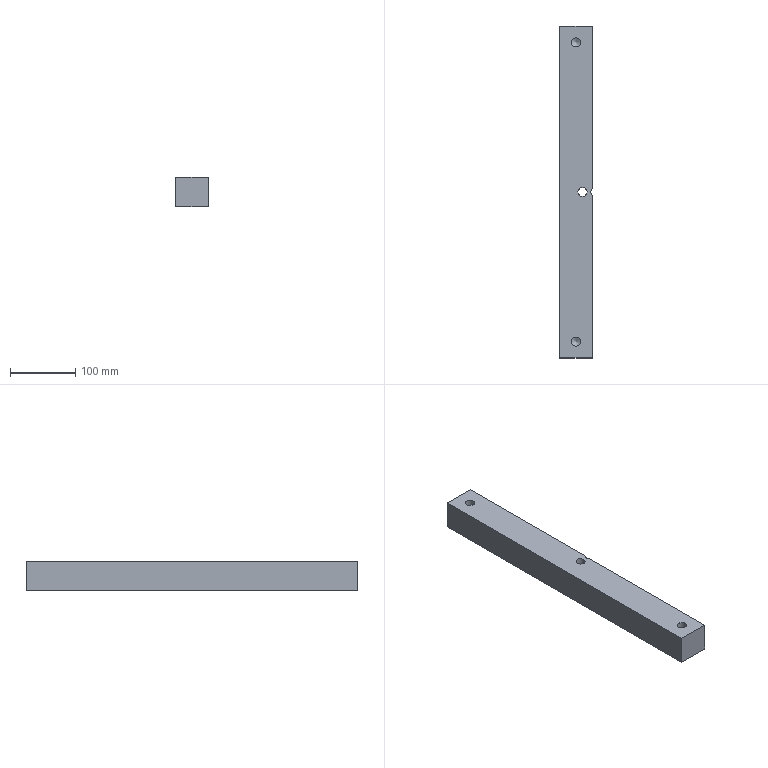Part | STEP file | 013_id2194_x_t | 1 solid | 13 faces | box 50 x 510 x 45 mm | volume 1133560 mm3 | plane 7 | cylinder 4 | cone 2 | commonest cylinder face diameters 14 x4
STEP:
#1=CARTESIAN_POINT('',(0.,0.,0.));
#2=DIRECTION('',(0.,0.,1.));
#3=DIRECTION('',(1.,0.,0.));
#4=AXIS2_PLACEMENT_3D('',#1,#2,#3);
#5=CARTESIAN_POINT('',(-701.5,-4.899,185.));
#6=VERTEX_POINT('',#5);
#7=CARTESIAN_POINT('',(-701.5,4.899,185.));
#8=VERTEX_POINT('',#7);
#9=CARTESIAN_POINT('',(-696.5,0.,185.));
#10=DIRECTION('',(0.,0.,-1.));
#11=DIRECTION('',(1.,0.,0.));
#12=AXIS2_PLACEMENT_3D('',#9,#10,#11);
#13=CIRCLE('',#12,7.);
#14=CARTESIAN_POINT('',(-751.5,-350.,185.));
#15=DIRECTION('',(0.,0.,1.));
#16=DIRECTION('',(0.,-1.,0.));
#17=AXIS2_PLACEMENT_3D('',#14,#15,#16);
#18=PLANE('',#17);
#19=CARTESIAN_POINT('',(-350.,62.));
#20=CARTESIAN_POINT('',(-337.876,62.));
#21=CARTESIAN_POINT('',(-343.938,51.5));
#22=CARTESIAN_POINT('',(-350.,41.));
#23=CARTESIAN_POINT('',(-356.062,51.5));
#24=CARTESIAN_POINT('',(-362.124,62.));
#25=CARTESIAN_POINT('',(-350.,62.));
#26=(BOUNDED_CURVE()B_SPLINE_CURVE(2,(#19,#20,#21,#22,#23,#24,#25),.UNSPECIFIED.,.T.,.F.)B_SPLINE_CURVE_WITH_KNOTS((1,2,2,2,2,1),(-2.094,0.,2.094,4.189,6.283,8.378),.UNSPECIFIED.)CURVE()GEOMETRIC_REPRESENTATION_ITEM()RATIONAL_B_SPLINE_CURVE((1.,0.5,1.,0.5,1.,0.5,1.))REPRESENTATION_ITEM(''));
#27=(GEOMETRIC_REPRESENTATION_CONTEXT(2)PARAMETRIC_REPRESENTATION_CONTEXT()REPRESENTATION_CONTEXT('',''));
#28=DEFINITIONAL_REPRESENTATION('',(#26),#27);
#29=PCURVE('',#18,#28);
#30=CARTESIAN_POINT('',(-696.5,0.,595.));
#31=DIRECTION('',(0.,0.,-1.));
#32=DIRECTION('',(-1.,0.,0.));
#33=AXIS2_PLACEMENT_3D('',#30,#31,#32);
#34=CYLINDRICAL_SURFACE('',#33,7.);
#35=CARTESIAN_POINT('',(-3.142,410.));
#36=DIRECTION('',(1.,0.));
#37=VECTOR('',#36,1.);
#38=LINE('',#35,#37);
#39=(GEOMETRIC_REPRESENTATION_CONTEXT(2)PARAMETRIC_REPRESENTATION_CONTEXT()REPRESENTATION_CONTEXT('',''));
#40=DEFINITIONAL_REPRESENTATION('',(#38),#39);
#41=PCURVE('',#34,#40);
#42=SURFACE_CURVE('',#13,(#29,#41),.PCURVE_S1.);
#43=EDGE_CURVE('',#6,#8,#42,.T.);
#44=ORIENTED_EDGE('',*,*,#43,.F.);
#45=CARTESIAN_POINT('',(-701.5,-255.,185.));
#46=VERTEX_POINT('',#45);
#47=CARTESIAN_POINT('',(-701.5,-350.,185.));
#48=DIRECTION('',(0.,1.,0.));
#49=VECTOR('',#48,1.);
#50=LINE('',#47,#49);
#51=CARTESIAN_POINT('',(0.,50.));
#52=DIRECTION('',(-1.,0.));
#53=VECTOR('',#52,1.);
#54=LINE('',#51,#53);
#55=(GEOMETRIC_REPRESENTATION_CONTEXT(2)PARAMETRIC_REPRESENTATION_CONTEXT()REPRESENTATION_CONTEXT('',''));
#56=DEFINITIONAL_REPRESENTATION('',(#54),#55);
#57=PCURVE('',#18,#56);
#58=CARTESIAN_POINT('',(-701.5,-350.,428.5));
#59=DIRECTION('',(-1.,0.,0.));
#60=DIRECTION('',(0.,0.,-1.));
#61=AXIS2_PLACEMENT_3D('',#58,#59,#60);
#62=PLANE('',#61);
#63=CARTESIAN_POINT('',(243.5,0.));
#64=DIRECTION('',(0.,-1.));
#65=VECTOR('',#64,1.);
#66=LINE('',#63,#65);
#67=(GEOMETRIC_REPRESENTATION_CONTEXT(2)PARAMETRIC_REPRESENTATION_CONTEXT()REPRESENTATION_CONTEXT('',''));
#68=DEFINITIONAL_REPRESENTATION('',(#66),#67);
#69=PCURVE('',#62,#68);
#70=SURFACE_CURVE('',#50,(#57,#69),.PCURVE_S1.);
#71=EDGE_CURVE('',#46,#6,#70,.T.);
#72=ORIENTED_EDGE('',*,*,#71,.F.);
#73=CARTESIAN_POINT('',(-751.5,-255.,185.));
#74=VERTEX_POINT('',#73);
#75=CARTESIAN_POINT('',(-751.5,-255.,185.));
#76=DIRECTION('',(-1.,0.,0.));
#77=VECTOR('',#76,1.);
#78=LINE('',#75,#77);
#79=CARTESIAN_POINT('',(-95.,0.));
#80=DIRECTION('',(0.,-1.));
#81=VECTOR('',#80,1.);
#82=LINE('',#79,#81);
#83=(GEOMETRIC_REPRESENTATION_CONTEXT(2)PARAMETRIC_REPRESENTATION_CONTEXT()REPRESENTATION_CONTEXT('',''));
#84=DEFINITIONAL_REPRESENTATION('',(#82),#83);
#85=PCURVE('',#18,#84);
#86=CARTESIAN_POINT('',(-751.5,-255.,428.5));
#87=DIRECTION('',(0.,1.,0.));
#88=DIRECTION('',(0.,0.,1.));
#89=AXIS2_PLACEMENT_3D('',#86,#87,#88);
#90=PLANE('',#89);
#91=CARTESIAN_POINT('',(-243.5,0.));
#92=DIRECTION('',(0.,-1.));
#93=VECTOR('',#92,1.);
#94=LINE('',#91,#93);
#95=(GEOMETRIC_REPRESENTATION_CONTEXT(2)PARAMETRIC_REPRESENTATION_CONTEXT()REPRESENTATION_CONTEXT('',''));
#96=DEFINITIONAL_REPRESENTATION('',(#94),#95);
#97=PCURVE('',#90,#96);
#98=SURFACE_CURVE('',#78,(#85,#97),.PCURVE_S1.);
#99=EDGE_CURVE('',#46,#74,#98,.T.);
#100=ORIENTED_EDGE('',*,*,#99,.T.);
#101=CARTESIAN_POINT('',(-751.5,255.,185.));
#102=VERTEX_POINT('',#101);
#103=CARTESIAN_POINT('',(-751.5,-350.,185.));
#104=DIRECTION('',(0.,1.,0.));
#105=VECTOR('',#104,1.);
#106=LINE('',#103,#105);
#107=CARTESIAN_POINT('',(0.,0.));
#108=DIRECTION('',(-1.,0.));
#109=VECTOR('',#108,1.);
#110=LINE('',#107,#109);
#111=(GEOMETRIC_REPRESENTATION_CONTEXT(2)PARAMETRIC_REPRESENTATION_CONTEXT()REPRESENTATION_CONTEXT('',''));
#112=DEFINITIONAL_REPRESENTATION('',(#110),#111);
#113=PCURVE('',#18,#112);
#114=CARTESIAN_POINT('',(-751.5,-350.,428.5));
#115=DIRECTION('',(-1.,0.,0.));
#116=DIRECTION('',(0.,0.,-1.));
#117=AXIS2_PLACEMENT_3D('',#114,#115,#116);
#118=PLANE('',#117);
#119=CARTESIAN_POINT('',(243.5,0.));
#120=DIRECTION('',(0.,-1.));
#121=VECTOR('',#120,1.);
#122=LINE('',#119,#121);
#123=(GEOMETRIC_REPRESENTATION_CONTEXT(2)PARAMETRIC_REPRESENTATION_CONTEXT()REPRESENTATION_CONTEXT('',''));
#124=DEFINITIONAL_REPRESENTATION('',(#122),#123);
#125=PCURVE('',#118,#124);
#126=SURFACE_CURVE('',#106,(#113,#125),.PCURVE_S1.);
#127=EDGE_CURVE('',#74,#102,#126,.T.);
#128=ORIENTED_EDGE('',*,*,#127,.T.);
#129=CARTESIAN_POINT('',(-701.5,255.,185.));
#130=VERTEX_POINT('',#129);
#131=CARTESIAN_POINT('',(-751.5,255.,185.));
#132=DIRECTION('',(-1.,0.,0.));
#133=VECTOR('',#132,1.);
#134=LINE('',#131,#133);
#135=CARTESIAN_POINT('',(-605.,0.));
#136=DIRECTION('',(0.,-1.));
#137=VECTOR('',#136,1.);
#138=LINE('',#135,#137);
#139=(GEOMETRIC_REPRESENTATION_CONTEXT(2)PARAMETRIC_REPRESENTATION_CONTEXT()REPRESENTATION_CONTEXT('',''));
#140=DEFINITIONAL_REPRESENTATION('',(#138),#139);
#141=PCURVE('',#18,#140);
#142=CARTESIAN_POINT('',(-751.5,255.,428.5));
#143=DIRECTION('',(0.,1.,0.));
#144=DIRECTION('',(0.,0.,1.));
#145=AXIS2_PLACEMENT_3D('',#142,#143,#144);
#146=PLANE('',#145);
#147=CARTESIAN_POINT('',(-243.5,0.));
#148=DIRECTION('',(0.,-1.));
#149=VECTOR('',#148,1.);
#150=LINE('',#147,#149);
#151=(GEOMETRIC_REPRESENTATION_CONTEXT(2)PARAMETRIC_REPRESENTATION_CONTEXT()REPRESENTATION_CONTEXT('',''));
#152=DEFINITIONAL_REPRESENTATION('',(#150),#151);
#153=PCURVE('',#146,#152);
#154=SURFACE_CURVE('',#134,(#141,#153),.PCURVE_S1.);
#155=EDGE_CURVE('',#130,#102,#154,.T.);
#156=ORIENTED_EDGE('',*,*,#155,.F.);
#157=CARTESIAN_POINT('',(-701.5,-350.,185.));
#158=DIRECTION('',(0.,1.,0.));
#159=VECTOR('',#158,1.);
#160=LINE('',#157,#159);
#161=CARTESIAN_POINT('',(0.,50.));
#162=DIRECTION('',(-1.,0.));
#163=VECTOR('',#162,1.);
#164=LINE('',#161,#163);
#165=(GEOMETRIC_REPRESENTATION_CONTEXT(2)PARAMETRIC_REPRESENTATION_CONTEXT()REPRESENTATION_CONTEXT('',''));
#166=DEFINITIONAL_REPRESENTATION('',(#164),#165);
#167=PCURVE('',#18,#166);
#168=CARTESIAN_POINT('',(-701.5,-350.,428.5));
#169=DIRECTION('',(-1.,0.,0.));
#170=DIRECTION('',(0.,0.,-1.));
#171=AXIS2_PLACEMENT_3D('',#168,#169,#170);
#172=PLANE('',#171);
#173=CARTESIAN_POINT('',(243.5,0.));
#174=DIRECTION('',(0.,-1.));
#175=VECTOR('',#174,1.);
#176=LINE('',#173,#175);
#177=(GEOMETRIC_REPRESENTATION_CONTEXT(2)PARAMETRIC_REPRESENTATION_CONTEXT()REPRESENTATION_CONTEXT('',''));
#178=DEFINITIONAL_REPRESENTATION('',(#176),#177);
#179=PCURVE('',#172,#178);
#180=SURFACE_CURVE('',#160,(#167,#179),.PCURVE_S1.);
#181=EDGE_CURVE('',#8,#130,#180,.T.);
#182=ORIENTED_EDGE('',*,*,#181,.F.);
#183=EDGE_LOOP('',(#44,#72,#100,#128,#156,#182));
#184=FACE_BOUND('',#183,.T.);
#185=CARTESIAN_POINT('',(-709.5,0.,185.));
#186=VERTEX_POINT('',#185);
#187=CARTESIAN_POINT('',(-716.5,0.,185.));
#188=DIRECTION('',(0.,0.,-1.));
#189=DIRECTION('',(1.,0.,0.));
#190=AXIS2_PLACEMENT_3D('',#187,#188,#189);
#191=CIRCLE('',#190,7.);
#192=CARTESIAN_POINT('',(-350.,42.));
#193=CARTESIAN_POINT('',(-337.876,42.));
#194=CARTESIAN_POINT('',(-343.938,31.5));
#195=CARTESIAN_POINT('',(-350.,21.));
#196=CARTESIAN_POINT('',(-356.062,31.5));
#197=CARTESIAN_POINT('',(-362.124,42.));
#198=CARTESIAN_POINT('',(-350.,42.));
#199=(BOUNDED_CURVE()B_SPLINE_CURVE(2,(#192,#193,#194,#195,#196,#197,#198),.UNSPECIFIED.,.T.,.F.)B_SPLINE_CURVE_WITH_KNOTS((1,2,2,2,2,1),(-2.094,0.,2.094,4.189,6.283,8.378),.UNSPECIFIED.)CURVE()GEOMETRIC_REPRESENTATION_ITEM()RATIONAL_B_SPLINE_CURVE((1.,0.5,1.,0.5,1.,0.5,1.))REPRESENTATION_ITEM(''));
#200=(GEOMETRIC_REPRESENTATION_CONTEXT(2)PARAMETRIC_REPRESENTATION_CONTEXT()REPRESENTATION_CONTEXT('',''));
#201=DEFINITIONAL_REPRESENTATION('',(#199),#200);
#202=PCURVE('',#18,#201);
#203=CARTESIAN_POINT('',(-716.5,0.,595.));
#204=DIRECTION('',(0.,0.,-1.));
#205=DIRECTION('',(-1.,0.,0.));
#206=AXIS2_PLACEMENT_3D('',#203,#204,#205);
#207=CYLINDRICAL_SURFACE('',#206,7.);
#208=CARTESIAN_POINT('',(3.142,410.));
#209=DIRECTION('',(1.,0.));
#210=VECTOR('',#209,1.);
#211=LINE('',#208,#210);
#212=(GEOMETRIC_REPRESENTATION_CONTEXT(2)PARAMETRIC_REPRESENTATION_CONTEXT()REPRESENTATION_CONTEXT('',''));
#213=DEFINITIONAL_REPRESENTATION('',(#211),#212);
#214=PCURVE('',#207,#213);
#215=SURFACE_CURVE('',#191,(#202,#214),.PCURVE_S1.);
#216=EDGE_CURVE('',#186,#186,#215,.T.);
#217=ORIENTED_EDGE('',*,*,#216,.F.);
#218=EDGE_LOOP('',(#217));
#219=FACE_BOUND('',#218,.T.);
#220=ADVANCED_FACE('',(#184,#219),#18,.F.);
#221=CARTESIAN_POINT('',(-701.5,4.899,230.));
#222=VERTEX_POINT('',#221);
#223=CARTESIAN_POINT('',(-701.5,255.,230.));
#224=VERTEX_POINT('',#223);
#225=CARTESIAN_POINT('',(-701.5,-350.,230.));
#226=DIRECTION('',(0.,1.,0.));
#227=VECTOR('',#226,1.);
#228=LINE('',#225,#227);
#229=CARTESIAN_POINT('',(198.5,0.));
#230=DIRECTION('',(0.,-1.));
#231=VECTOR('',#230,1.);
#232=LINE('',#229,#231);
#233=(GEOMETRIC_REPRESENTATION_CONTEXT(2)PARAMETRIC_REPRESENTATION_CONTEXT()REPRESENTATION_CONTEXT('',''));
#234=DEFINITIONAL_REPRESENTATION('',(#232),#233);
#235=PCURVE('',#172,#234);
#236=CARTESIAN_POINT('',(-546.5,-140.,230.));
#237=DIRECTION('',(0.,0.,1.));
#238=DIRECTION('',(1.,0.,0.));
#239=AXIS2_PLACEMENT_3D('',#236,#237,#238);
#240=PLANE('',#239);
#241=CARTESIAN_POINT('',(-155.,-210.));
#242=DIRECTION('',(0.,1.));
#243=VECTOR('',#242,1.);
#244=LINE('',#241,#243);
#245=(GEOMETRIC_REPRESENTATION_CONTEXT(2)PARAMETRIC_REPRESENTATION_CONTEXT()REPRESENTATION_CONTEXT('',''));
#246=DEFINITIONAL_REPRESENTATION('',(#244),#245);
#247=PCURVE('',#240,#246);
#248=SURFACE_CURVE('',#228,(#235,#247),.PCURVE_S1.);
#249=EDGE_CURVE('',#222,#224,#248,.T.);
#250=ORIENTED_EDGE('',*,*,#249,.F.);
#251=CARTESIAN_POINT('',(-701.5,4.899,595.));
#252=DIRECTION('',(0.,0.,-1.));
#253=VECTOR('',#252,1.);
#254=LINE('',#251,#253);
#255=CARTESIAN_POINT('',(-166.5,-354.899));
#256=DIRECTION('',(1.,0.));
#257=VECTOR('',#256,1.);
#258=LINE('',#255,#257);
#259=(GEOMETRIC_REPRESENTATION_CONTEXT(2)PARAMETRIC_REPRESENTATION_CONTEXT()REPRESENTATION_CONTEXT('',''));
#260=DEFINITIONAL_REPRESENTATION('',(#258),#259);
#261=PCURVE('',#172,#260);
#262=CARTESIAN_POINT('',(0.7752,0.));
#263=DIRECTION('',(0.,1.));
#264=VECTOR('',#263,1.);
#265=LINE('',#262,#264);
#266=(GEOMETRIC_REPRESENTATION_CONTEXT(2)PARAMETRIC_REPRESENTATION_CONTEXT()REPRESENTATION_CONTEXT('',''));
#267=DEFINITIONAL_REPRESENTATION('',(#265),#266);
#268=PCURVE('',#34,#267);
#269=SURFACE_CURVE('',#254,(#261,#268),.PCURVE_S1.);
#270=EDGE_CURVE('',#222,#8,#269,.T.);
#271=ORIENTED_EDGE('',*,*,#270,.T.);
#272=ORIENTED_EDGE('',*,*,#181,.T.);
#273=CARTESIAN_POINT('',(-701.5,255.,428.5));
#274=DIRECTION('',(0.,0.,1.));
#275=VECTOR('',#274,1.);
#276=LINE('',#273,#275);
#277=CARTESIAN_POINT('',(0.,-605.));
#278=DIRECTION('',(-1.,0.));
#279=VECTOR('',#278,1.);
#280=LINE('',#277,#279);
#281=(GEOMETRIC_REPRESENTATION_CONTEXT(2)PARAMETRIC_REPRESENTATION_CONTEXT()REPRESENTATION_CONTEXT('',''));
#282=DEFINITIONAL_REPRESENTATION('',(#280),#281);
#283=PCURVE('',#172,#282);
#284=CARTESIAN_POINT('',(0.,50.));
#285=DIRECTION('',(1.,0.));
#286=VECTOR('',#285,1.);
#287=LINE('',#284,#286);
#288=(GEOMETRIC_REPRESENTATION_CONTEXT(2)PARAMETRIC_REPRESENTATION_CONTEXT()REPRESENTATION_CONTEXT('',''));
#289=DEFINITIONAL_REPRESENTATION('',(#287),#288);
#290=PCURVE('',#146,#289);
#291=SURFACE_CURVE('',#276,(#283,#290),.PCURVE_S1.);
#292=EDGE_CURVE('',#130,#224,#291,.T.);
#293=ORIENTED_EDGE('',*,*,#292,.T.);
#294=EDGE_LOOP('',(#250,#271,#272,#293));
#295=FACE_BOUND('',#294,.T.);
#296=ADVANCED_FACE('',(#295),#172,.F.);
#297=CARTESIAN_POINT('',(-709.5,0.,230.));
#298=VERTEX_POINT('',#297);
#299=CARTESIAN_POINT('',(-716.5,0.,230.));
#300=DIRECTION('',(0.,0.,1.));
#301=DIRECTION('',(1.,0.,0.));
#302=AXIS2_PLACEMENT_3D('',#299,#300,#301);
#303=CIRCLE('',#302,7.);
#304=CARTESIAN_POINT('',(-170.,140.));
#305=DIRECTION('',(1.,0.));
#306=AXIS2_PLACEMENT_2D('',#304,#305);
#307=CIRCLE('',#306,7.);
#308=(GEOMETRIC_REPRESENTATION_CONTEXT(2)PARAMETRIC_REPRESENTATION_CONTEXT()REPRESENTATION_CONTEXT('',''));
#309=DEFINITIONAL_REPRESENTATION('',(#307),#308);
#310=PCURVE('',#240,#309);
#311=CARTESIAN_POINT('',(9.425,365.));
#312=DIRECTION('',(-1.,0.));
#313=VECTOR('',#312,1.);
#314=LINE('',#311,#313);
#315=(GEOMETRIC_REPRESENTATION_CONTEXT(2)PARAMETRIC_REPRESENTATION_CONTEXT()REPRESENTATION_CONTEXT('',''));
#316=DEFINITIONAL_REPRESENTATION('',(#314),#315);
#317=PCURVE('',#207,#316);
#318=SURFACE_CURVE('',#303,(#310,#317),.PCURVE_S1.);
#319=EDGE_CURVE('',#298,#298,#318,.T.);
#320=ORIENTED_EDGE('',*,*,#319,.F.);
#321=EDGE_LOOP('',(#320));
#322=FACE_BOUND('',#321,.T.);
#323=CARTESIAN_POINT('',(-701.5,-4.899,230.));
#324=VERTEX_POINT('',#323);
#325=CARTESIAN_POINT('',(-696.5,0.,230.));
#326=DIRECTION('',(0.,0.,1.));
#327=DIRECTION('',(1.,0.,0.));
#328=AXIS2_PLACEMENT_3D('',#325,#326,#327);
#329=CIRCLE('',#328,7.);
#330=CARTESIAN_POINT('',(-150.,140.));
#331=DIRECTION('',(1.,0.));
#332=AXIS2_PLACEMENT_2D('',#330,#331);
#333=CIRCLE('',#332,7.);
#334=(GEOMETRIC_REPRESENTATION_CONTEXT(2)PARAMETRIC_REPRESENTATION_CONTEXT()REPRESENTATION_CONTEXT('',''));
#335=DEFINITIONAL_REPRESENTATION('',(#333),#334);
#336=PCURVE('',#240,#335);
#337=CARTESIAN_POINT('',(3.142,365.));
#338=DIRECTION('',(-1.,0.));
#339=VECTOR('',#338,1.);
#340=LINE('',#337,#339);
#341=(GEOMETRIC_REPRESENTATION_CONTEXT(2)PARAMETRIC_REPRESENTATION_CONTEXT()REPRESENTATION_CONTEXT('',''));
#342=DEFINITIONAL_REPRESENTATION('',(#340),#341);
#343=PCURVE('',#34,#342);
#344=SURFACE_CURVE('',#329,(#336,#343),.PCURVE_S1.);
#345=EDGE_CURVE('',#222,#324,#344,.T.);
#346=ORIENTED_EDGE('',*,*,#345,.F.);
#347=ORIENTED_EDGE('',*,*,#249,.T.);
#348=CARTESIAN_POINT('',(-751.5,255.,230.));
#349=VERTEX_POINT('',#348);
#350=CARTESIAN_POINT('',(-751.5,255.,230.));
#351=DIRECTION('',(-1.,0.,0.));
#352=VECTOR('',#351,1.);
#353=LINE('',#350,#352);
#354=CARTESIAN_POINT('',(-205.,395.));
#355=DIRECTION('',(-1.,0.));
#356=VECTOR('',#355,1.);
#357=LINE('',#354,#356);
#358=(GEOMETRIC_REPRESENTATION_CONTEXT(2)PARAMETRIC_REPRESENTATION_CONTEXT()REPRESENTATION_CONTEXT('',''));
#359=DEFINITIONAL_REPRESENTATION('',(#357),#358);
#360=PCURVE('',#240,#359);
#361=CARTESIAN_POINT('',(-198.5,0.));
#362=DIRECTION('',(0.,-1.));
#363=VECTOR('',#362,1.);
#364=LINE('',#361,#363);
#365=(GEOMETRIC_REPRESENTATION_CONTEXT(2)PARAMETRIC_REPRESENTATION_CONTEXT()REPRESENTATION_CONTEXT('',''));
#366=DEFINITIONAL_REPRESENTATION('',(#364),#365);
#367=PCURVE('',#146,#366);
#368=SURFACE_CURVE('',#353,(#360,#367),.PCURVE_S1.);
#369=EDGE_CURVE('',#224,#349,#368,.T.);
#370=ORIENTED_EDGE('',*,*,#369,.T.);
#371=CARTESIAN_POINT('',(-751.5,-255.,230.));
#372=VERTEX_POINT('',#371);
#373=CARTESIAN_POINT('',(-751.5,-350.,230.));
#374=DIRECTION('',(0.,-1.,0.));
#375=VECTOR('',#374,1.);
#376=LINE('',#373,#375);
#377=CARTESIAN_POINT('',(-205.,-210.));
#378=DIRECTION('',(0.,-1.));
#379=VECTOR('',#378,1.);
#380=LINE('',#377,#379);
#381=(GEOMETRIC_REPRESENTATION_CONTEXT(2)PARAMETRIC_REPRESENTATION_CONTEXT()REPRESENTATION_CONTEXT('',''));
#382=DEFINITIONAL_REPRESENTATION('',(#380),#381);
#383=PCURVE('',#240,#382);
#384=CARTESIAN_POINT('',(198.5,0.));
#385=DIRECTION('',(0.,1.));
#386=VECTOR('',#385,1.);
#387=LINE('',#384,#386);
#388=(GEOMETRIC_REPRESENTATION_CONTEXT(2)PARAMETRIC_REPRESENTATION_CONTEXT()REPRESENTATION_CONTEXT('',''));
#389=DEFINITIONAL_REPRESENTATION('',(#387),#388);
#390=PCURVE('',#118,#389);
#391=SURFACE_CURVE('',#376,(#383,#390),.PCURVE_S1.);
#392=EDGE_CURVE('',#349,#372,#391,.T.);
#393=ORIENTED_EDGE('',*,*,#392,.T.);
#394=CARTESIAN_POINT('',(-701.5,-255.,230.));
#395=VERTEX_POINT('',#394);
#396=CARTESIAN_POINT('',(-751.5,-255.,230.));
#397=DIRECTION('',(-1.,0.,0.));
#398=VECTOR('',#397,1.);
#399=LINE('',#396,#398);
#400=CARTESIAN_POINT('',(-205.,-115.));
#401=DIRECTION('',(-1.,0.));
#402=VECTOR('',#401,1.);
#403=LINE('',#400,#402);
#404=(GEOMETRIC_REPRESENTATION_CONTEXT(2)PARAMETRIC_REPRESENTATION_CONTEXT()REPRESENTATION_CONTEXT('',''));
#405=DEFINITIONAL_REPRESENTATION('',(#403),#404);
#406=PCURVE('',#240,#405);
#407=CARTESIAN_POINT('',(-198.5,0.));
#408=DIRECTION('',(0.,-1.));
#409=VECTOR('',#408,1.);
#410=LINE('',#407,#409);
#411=(GEOMETRIC_REPRESENTATION_CONTEXT(2)PARAMETRIC_REPRESENTATION_CONTEXT()REPRESENTATION_CONTEXT('',''));
#412=DEFINITIONAL_REPRESENTATION('',(#410),#411);
#413=PCURVE('',#90,#412);
#414=SURFACE_CURVE('',#399,(#406,#413),.PCURVE_S1.);
#415=EDGE_CURVE('',#395,#372,#414,.T.);
#416=ORIENTED_EDGE('',*,*,#415,.F.);
#417=CARTESIAN_POINT('',(-701.5,-350.,230.));
#418=DIRECTION('',(0.,1.,0.));
#419=VECTOR('',#418,1.);
#420=LINE('',#417,#419);
#421=CARTESIAN_POINT('',(-155.,-210.));
#422=DIRECTION('',(0.,1.));
#423=VECTOR('',#422,1.);
#424=LINE('',#421,#423);
#425=(GEOMETRIC_REPRESENTATION_CONTEXT(2)PARAMETRIC_REPRESENTATION_CONTEXT()REPRESENTATION_CONTEXT('',''));
#426=DEFINITIONAL_REPRESENTATION('',(#424),#425);
#427=PCURVE('',#240,#426);
#428=CARTESIAN_POINT('',(198.5,0.));
#429=DIRECTION('',(0.,-1.));
#430=VECTOR('',#429,1.);
#431=LINE('',#428,#430);
#432=(GEOMETRIC_REPRESENTATION_CONTEXT(2)PARAMETRIC_REPRESENTATION_CONTEXT()REPRESENTATION_CONTEXT('',''));
#433=DEFINITIONAL_REPRESENTATION('',(#431),#432);
#434=PCURVE('',#62,#433);
#435=SURFACE_CURVE('',#420,(#427,#434),.PCURVE_S1.);
#436=EDGE_CURVE('',#395,#324,#435,.T.);
#437=ORIENTED_EDGE('',*,*,#436,.T.);
#438=EDGE_LOOP('',(#346,#347,#370,#393,#416,#437));
#439=FACE_BOUND('',#438,.T.);
#440=CARTESIAN_POINT('',(-733.5,230.,230.));
#441=VERTEX_POINT('',#440);
#442=CARTESIAN_POINT('',(-719.5,230.,230.));
#443=VERTEX_POINT('',#442);
#444=CARTESIAN_POINT('',(-726.5,230.,230.));
#445=DIRECTION('',(0.,0.,1.));
#446=DIRECTION('',(-1.,0.,0.));
#447=AXIS2_PLACEMENT_3D('',#444,#445,#446);
#448=CIRCLE('',#447,7.);
#449=CARTESIAN_POINT('',(-180.,370.));
#450=DIRECTION('',(-1.,0.));
#451=AXIS2_PLACEMENT_2D('',#449,#450);
#452=CIRCLE('',#451,7.);
#453=(GEOMETRIC_REPRESENTATION_CONTEXT(2)PARAMETRIC_REPRESENTATION_CONTEXT()REPRESENTATION_CONTEXT('',''));
#454=DEFINITIONAL_REPRESENTATION('',(#452),#453);
#455=PCURVE('',#240,#454);
#456=CARTESIAN_POINT('',(-726.5,230.,279.));
#457=DIRECTION('',(0.,0.,-1.));
#458=DIRECTION('',(1.,0.,0.));
#459=AXIS2_PLACEMENT_3D('',#456,#457,#458);
#460=CYLINDRICAL_SURFACE('',#459,7.);
#461=CARTESIAN_POINT('',(3.142,49.));
#462=DIRECTION('',(-1.,0.));
#463=VECTOR('',#462,1.);
#464=LINE('',#461,#463);
#465=(GEOMETRIC_REPRESENTATION_CONTEXT(2)PARAMETRIC_REPRESENTATION_CONTEXT()REPRESENTATION_CONTEXT('',''));
#466=DEFINITIONAL_REPRESENTATION('',(#464),#465);
#467=PCURVE('',#460,#466);
#468=SURFACE_CURVE('',#448,(#455,#467),.PCURVE_S1.);
#469=EDGE_CURVE('',#441,#443,#468,.T.);
#470=ORIENTED_EDGE('',*,*,#469,.F.);
#471=CARTESIAN_POINT('',(-726.5,230.,230.));
#472=DIRECTION('',(0.,0.,1.));
#473=DIRECTION('',(-1.,0.,0.));
#474=AXIS2_PLACEMENT_3D('',#471,#472,#473);
#475=CIRCLE('',#474,7.);
#476=CARTESIAN_POINT('',(-180.,370.));
#477=DIRECTION('',(-1.,0.));
#478=AXIS2_PLACEMENT_2D('',#476,#477);
#479=CIRCLE('',#478,7.);
#480=(GEOMETRIC_REPRESENTATION_CONTEXT(2)PARAMETRIC_REPRESENTATION_CONTEXT()REPRESENTATION_CONTEXT('',''));
#481=DEFINITIONAL_REPRESENTATION('',(#479),#480);
#482=PCURVE('',#240,#481);
#483=CARTESIAN_POINT('',(9.425,49.));
#484=DIRECTION('',(-1.,0.));
#485=VECTOR('',#484,1.);
#486=LINE('',#483,#485);
#487=(GEOMETRIC_REPRESENTATION_CONTEXT(2)PARAMETRIC_REPRESENTATION_CONTEXT()REPRESENTATION_CONTEXT('',''));
#488=DEFINITIONAL_REPRESENTATION('',(#486),#487);
#489=PCURVE('',#460,#488);
#490=SURFACE_CURVE('',#475,(#482,#489),.PCURVE_S1.);
#491=EDGE_CURVE('',#443,#441,#490,.T.);
#492=ORIENTED_EDGE('',*,*,#491,.F.);
#493=EDGE_LOOP('',(#470,#492));
#494=FACE_BOUND('',#493,.T.);
#495=CARTESIAN_POINT('',(-733.5,-230.,230.));
#496=VERTEX_POINT('',#495);
#497=CARTESIAN_POINT('',(-719.5,-230.,230.));
#498=VERTEX_POINT('',#497);
#499=CARTESIAN_POINT('',(-726.5,-230.,230.));
#500=DIRECTION('',(0.,0.,-1.));
#501=DIRECTION('',(-1.,0.,0.));
#502=AXIS2_PLACEMENT_3D('',#499,#500,#501);
#503=CIRCLE('',#502,7.);
#504=CARTESIAN_POINT('',(-187.,-90.));
#505=CARTESIAN_POINT('',(-187.,-77.876));
#506=CARTESIAN_POINT('',(-176.5,-83.938));
#507=CARTESIAN_POINT('',(-166.,-90.));
#508=CARTESIAN_POINT('',(-176.5,-96.062));
#509=CARTESIAN_POINT('',(-187.,-102.124));
#510=CARTESIAN_POINT('',(-187.,-90.));
#511=(BOUNDED_CURVE()B_SPLINE_CURVE(2,(#504,#505,#506,#507,#508,#509,#510),.UNSPECIFIED.,.T.,.F.)B_SPLINE_CURVE_WITH_KNOTS((1,2,2,2,2,1),(-2.094,0.,2.094,4.189,6.283,8.378),.UNSPECIFIED.)CURVE()GEOMETRIC_REPRESENTATION_ITEM()RATIONAL_B_SPLINE_CURVE((1.,0.5,1.,0.5,1.,0.5,1.))REPRESENTATION_ITEM(''));
#512=(GEOMETRIC_REPRESENTATION_CONTEXT(2)PARAMETRIC_REPRESENTATION_CONTEXT()REPRESENTATION_CONTEXT('',''));
#513=DEFINITIONAL_REPRESENTATION('',(#511),#512);
#514=PCURVE('',#240,#513);
#515=CARTESIAN_POINT('',(-726.5,-230.,279.));
#516=DIRECTION('',(0.,0.,-1.));
#517=DIRECTION('',(1.,0.,0.));
#518=AXIS2_PLACEMENT_3D('',#515,#516,#517);
#519=CYLINDRICAL_SURFACE('',#518,7.);
#520=CARTESIAN_POINT('',(3.142,49.));
#521=DIRECTION('',(1.,0.));
#522=VECTOR('',#521,1.);
#523=LINE('',#520,#522);
#524=(GEOMETRIC_REPRESENTATION_CONTEXT(2)PARAMETRIC_REPRESENTATION_CONTEXT()REPRESENTATION_CONTEXT('',''));
#525=DEFINITIONAL_REPRESENTATION('',(#523),#524);
#526=PCURVE('',#519,#525);
#527=SURFACE_CURVE('',#503,(#514,#526),.PCURVE_S1.);
#528=EDGE_CURVE('',#496,#498,#527,.T.);
#529=ORIENTED_EDGE('',*,*,#528,.T.);
#530=CARTESIAN_POINT('',(-726.5,-230.,230.));
#531=DIRECTION('',(0.,0.,-1.));
#532=DIRECTION('',(-1.,0.,0.));
#533=AXIS2_PLACEMENT_3D('',#530,#531,#532);
#534=CIRCLE('',#533,7.);
#535=CARTESIAN_POINT('',(-187.,-90.));
#536=CARTESIAN_POINT('',(-187.,-77.876));
#537=CARTESIAN_POINT('',(-176.5,-83.938));
#538=CARTESIAN_POINT('',(-166.,-90.));
#539=CARTESIAN_POINT('',(-176.5,-96.062));
#540=CARTESIAN_POINT('',(-187.,-102.124));
#541=CARTESIAN_POINT('',(-187.,-90.));
#542=(BOUNDED_CURVE()B_SPLINE_CURVE(2,(#535,#536,#537,#538,#539,#540,#541),.UNSPECIFIED.,.T.,.F.)B_SPLINE_CURVE_WITH_KNOTS((1,2,2,2,2,1),(-2.094,0.,2.094,4.189,6.283,8.378),.UNSPECIFIED.)CURVE()GEOMETRIC_REPRESENTATION_ITEM()RATIONAL_B_SPLINE_CURVE((1.,0.5,1.,0.5,1.,0.5,1.))REPRESENTATION_ITEM(''));
#543=(GEOMETRIC_REPRESENTATION_CONTEXT(2)PARAMETRIC_REPRESENTATION_CONTEXT()REPRESENTATION_CONTEXT('',''));
#544=DEFINITIONAL_REPRESENTATION('',(#542),#543);
#545=PCURVE('',#240,#544);
#546=CARTESIAN_POINT('',(-3.142,49.));
#547=DIRECTION('',(1.,0.));
#548=VECTOR('',#547,1.);
#549=LINE('',#546,#548);
#550=(GEOMETRIC_REPRESENTATION_CONTEXT(2)PARAMETRIC_REPRESENTATION_CONTEXT()REPRESENTATION_CONTEXT('',''));
#551=DEFINITIONAL_REPRESENTATION('',(#549),#550);
#552=PCURVE('',#519,#551);
#553=SURFACE_CURVE('',#534,(#545,#552),.PCURVE_S1.);
#554=EDGE_CURVE('',#498,#496,#553,.T.);
#555=ORIENTED_EDGE('',*,*,#554,.T.);
#556=EDGE_LOOP('',(#529,#555));
#557=FACE_BOUND('',#556,.T.);
#558=ADVANCED_FACE('',(#322,#439,#494,#557),#240,.T.);
#559=ORIENTED_EDGE('',*,*,#71,.T.);
#560=CARTESIAN_POINT('',(-701.5,-4.899,595.));
#561=DIRECTION('',(0.,0.,1.));
#562=VECTOR('',#561,1.);
#563=LINE('',#560,#562);
#564=CARTESIAN_POINT('',(-166.5,-345.101));
#565=DIRECTION('',(-1.,0.));
#566=VECTOR('',#565,1.);
#567=LINE('',#564,#566);
#568=(GEOMETRIC_REPRESENTATION_CONTEXT(2)PARAMETRIC_REPRESENTATION_CONTEXT()REPRESENTATION_CONTEXT('',''));
#569=DEFINITIONAL_REPRESENTATION('',(#567),#568);
#570=PCURVE('',#62,#569);
#571=CARTESIAN_POINT('',(-0.7752,0.));
#572=DIRECTION('',(0.,-1.));
#573=VECTOR('',#572,1.);
#574=LINE('',#571,#573);
#575=(GEOMETRIC_REPRESENTATION_CONTEXT(2)PARAMETRIC_REPRESENTATION_CONTEXT()REPRESENTATION_CONTEXT('',''));
#576=DEFINITIONAL_REPRESENTATION('',(#574),#575);
#577=PCURVE('',#34,#576);
#578=SURFACE_CURVE('',#563,(#570,#577),.PCURVE_S1.);
#579=EDGE_CURVE('',#6,#324,#578,.T.);
#580=ORIENTED_EDGE('',*,*,#579,.T.);
#581=ORIENTED_EDGE('',*,*,#436,.F.);
#582=CARTESIAN_POINT('',(-701.5,-255.,428.5));
#583=DIRECTION('',(0.,0.,-1.));
#584=VECTOR('',#583,1.);
#585=LINE('',#582,#584);
#586=CARTESIAN_POINT('',(0.,-95.));
#587=DIRECTION('',(1.,0.));
#588=VECTOR('',#587,1.);
#589=LINE('',#586,#588);
#590=(GEOMETRIC_REPRESENTATION_CONTEXT(2)PARAMETRIC_REPRESENTATION_CONTEXT()REPRESENTATION_CONTEXT('',''));
#591=DEFINITIONAL_REPRESENTATION('',(#589),#590);
#592=PCURVE('',#62,#591);
#593=CARTESIAN_POINT('',(0.,50.));
#594=DIRECTION('',(-1.,0.));
#595=VECTOR('',#594,1.);
#596=LINE('',#593,#595);
#597=(GEOMETRIC_REPRESENTATION_CONTEXT(2)PARAMETRIC_REPRESENTATION_CONTEXT()REPRESENTATION_CONTEXT('',''));
#598=DEFINITIONAL_REPRESENTATION('',(#596),#597);
#599=PCURVE('',#90,#598);
#600=SURFACE_CURVE('',#585,(#592,#599),.PCURVE_S1.);
#601=EDGE_CURVE('',#395,#46,#600,.T.);
#602=ORIENTED_EDGE('',*,*,#601,.T.);
#603=EDGE_LOOP('',(#559,#580,#581,#602));
#604=FACE_BOUND('',#603,.T.);
#605=ADVANCED_FACE('',(#604),#62,.F.);
#606=ORIENTED_EDGE('',*,*,#415,.T.);
#607=CARTESIAN_POINT('',(-751.5,-255.,428.5));
#608=DIRECTION('',(0.,0.,-1.));
#609=VECTOR('',#608,1.);
#610=LINE('',#607,#609);
#611=CARTESIAN_POINT('',(0.,0.));
#612=DIRECTION('',(-1.,0.));
#613=VECTOR('',#612,1.);
#614=LINE('',#611,#613);
#615=(GEOMETRIC_REPRESENTATION_CONTEXT(2)PARAMETRIC_REPRESENTATION_CONTEXT()REPRESENTATION_CONTEXT('',''));
#616=DEFINITIONAL_REPRESENTATION('',(#614),#615);
#617=PCURVE('',#90,#616);
#618=CARTESIAN_POINT('',(0.,-95.));
#619=DIRECTION('',(1.,0.));
#620=VECTOR('',#619,1.);
#621=LINE('',#618,#620);
#622=(GEOMETRIC_REPRESENTATION_CONTEXT(2)PARAMETRIC_REPRESENTATION_CONTEXT()REPRESENTATION_CONTEXT('',''));
#623=DEFINITIONAL_REPRESENTATION('',(#621),#622);
#624=PCURVE('',#118,#623);
#625=SURFACE_CURVE('',#610,(#617,#624),.PCURVE_S1.);
#626=EDGE_CURVE('',#372,#74,#625,.T.);
#627=ORIENTED_EDGE('',*,*,#626,.T.);
#628=ORIENTED_EDGE('',*,*,#99,.F.);
#629=ORIENTED_EDGE('',*,*,#601,.F.);
#630=EDGE_LOOP('',(#606,#627,#628,#629));
#631=FACE_BOUND('',#630,.T.);
#632=ADVANCED_FACE('',(#631),#90,.F.);
#633=CARTESIAN_POINT('',(-751.5,255.,428.5));
#634=DIRECTION('',(0.,0.,1.));
#635=VECTOR('',#634,1.);
#636=LINE('',#633,#635);
#637=CARTESIAN_POINT('',(0.,-605.));
#638=DIRECTION('',(-1.,0.));
#639=VECTOR('',#638,1.);
#640=LINE('',#637,#639);
#641=(GEOMETRIC_REPRESENTATION_CONTEXT(2)PARAMETRIC_REPRESENTATION_CONTEXT()REPRESENTATION_CONTEXT('',''));
#642=DEFINITIONAL_REPRESENTATION('',(#640),#641);
#643=PCURVE('',#118,#642);
#644=CARTESIAN_POINT('',(0.,0.));
#645=DIRECTION('',(1.,0.));
#646=VECTOR('',#645,1.);
#647=LINE('',#644,#646);
#648=(GEOMETRIC_REPRESENTATION_CONTEXT(2)PARAMETRIC_REPRESENTATION_CONTEXT()REPRESENTATION_CONTEXT('',''));
#649=DEFINITIONAL_REPRESENTATION('',(#647),#648);
#650=PCURVE('',#146,#649);
#651=SURFACE_CURVE('',#636,(#643,#650),.PCURVE_S1.);
#652=EDGE_CURVE('',#102,#349,#651,.T.);
#653=ORIENTED_EDGE('',*,*,#652,.F.);
#654=ORIENTED_EDGE('',*,*,#127,.F.);
#655=ORIENTED_EDGE('',*,*,#626,.F.);
#656=ORIENTED_EDGE('',*,*,#392,.F.);
#657=EDGE_LOOP('',(#653,#654,#655,#656));
#658=FACE_BOUND('',#657,.T.);
#659=ADVANCED_FACE('',(#658),#118,.T.);
#660=ORIENTED_EDGE('',*,*,#292,.F.);
#661=ORIENTED_EDGE('',*,*,#155,.T.);
#662=ORIENTED_EDGE('',*,*,#652,.T.);
#663=ORIENTED_EDGE('',*,*,#369,.F.);
#664=EDGE_LOOP('',(#660,#661,#662,#663));
#665=FACE_BOUND('',#664,.T.);
#666=ADVANCED_FACE('',(#665),#146,.T.);
#667=ORIENTED_EDGE('',*,*,#491,.F.);
#668=CARTESIAN_POINT('',(-719.5,230.,210.541));
#669=VERTEX_POINT('',#668);
#670=CARTESIAN_POINT('',(-719.5,230.,230.));
#671=CARTESIAN_POINT('',(-719.5,230.,210.541));
#672=B_SPLINE_CURVE_WITH_KNOTS('',1,(#670,#671),.UNSPECIFIED.,.F.,.F.,(2,2),(49.,68.459),.PIECEWISE_BEZIER_KNOTS.);
#673=CARTESIAN_POINT('',(6.283,0.));
#674=DIRECTION('',(0.,1.));
#675=VECTOR('',#674,1.);
#676=LINE('',#673,#675);
#677=(GEOMETRIC_REPRESENTATION_CONTEXT(2)PARAMETRIC_REPRESENTATION_CONTEXT()REPRESENTATION_CONTEXT('',''));
#678=DEFINITIONAL_REPRESENTATION('',(#676),#677);
#679=PCURVE('',#460,#678);
#680=CARTESIAN_POINT('',(0.,0.));
#681=DIRECTION('',(0.,1.));
#682=VECTOR('',#681,1.);
#683=LINE('',#680,#682);
#684=(GEOMETRIC_REPRESENTATION_CONTEXT(2)PARAMETRIC_REPRESENTATION_CONTEXT()REPRESENTATION_CONTEXT('',''));
#685=DEFINITIONAL_REPRESENTATION('',(#683),#684);
#686=PCURVE('',#460,#685);
#687=SEAM_CURVE('',#672,(#679,#686),.PCURVE_S1.);
#688=EDGE_CURVE('',#443,#669,#687,.T.);
#689=ORIENTED_EDGE('',*,*,#688,.T.);
#690=CARTESIAN_POINT('',(-733.5,230.,210.541));
#691=VERTEX_POINT('',#690);
#692=CARTESIAN_POINT('',(-726.5,230.,210.541));
#693=DIRECTION('',(0.,0.,1.));
#694=DIRECTION('',(1.,0.,0.));
#695=AXIS2_PLACEMENT_3D('',#692,#693,#694);
#696=CIRCLE('',#695,7.);
#697=CARTESIAN_POINT('',(6.283,68.459));
#698=DIRECTION('',(-1.,0.));
#699=VECTOR('',#698,1.);
#700=LINE('',#697,#699);
#701=(GEOMETRIC_REPRESENTATION_CONTEXT(2)PARAMETRIC_REPRESENTATION_CONTEXT()REPRESENTATION_CONTEXT('',''));
#702=DEFINITIONAL_REPRESENTATION('',(#700),#701);
#703=PCURVE('',#460,#702);
#704=CARTESIAN_POINT('',(-726.5,230.,210.541));
#705=DIRECTION('',(0.,0.,1.));
#706=DIRECTION('',(-1.,0.,0.));
#707=AXIS2_PLACEMENT_3D('',#704,#705,#706);
#708=CONICAL_SURFACE('',#707,7.,1.047);
#709=CARTESIAN_POINT('',(3.142,0.));
#710=DIRECTION('',(1.,0.));
#711=VECTOR('',#710,1.);
#712=LINE('',#709,#711);
#713=(GEOMETRIC_REPRESENTATION_CONTEXT(2)PARAMETRIC_REPRESENTATION_CONTEXT()REPRESENTATION_CONTEXT('',''));
#714=DEFINITIONAL_REPRESENTATION('',(#712),#713);
#715=PCURVE('',#708,#714);
#716=SURFACE_CURVE('',#696,(#703,#715),.PCURVE_S1.);
#717=EDGE_CURVE('',#669,#691,#716,.T.);
#718=ORIENTED_EDGE('',*,*,#717,.T.);
#719=CARTESIAN_POINT('',(-726.5,230.,210.541));
#720=DIRECTION('',(0.,0.,1.));
#721=DIRECTION('',(1.,0.,0.));
#722=AXIS2_PLACEMENT_3D('',#719,#720,#721);
#723=CIRCLE('',#722,7.);
#724=CARTESIAN_POINT('',(6.283,68.459));
#725=DIRECTION('',(-1.,0.));
#726=VECTOR('',#725,1.);
#727=LINE('',#724,#726);
#728=(GEOMETRIC_REPRESENTATION_CONTEXT(2)PARAMETRIC_REPRESENTATION_CONTEXT()REPRESENTATION_CONTEXT('',''));
#729=DEFINITIONAL_REPRESENTATION('',(#727),#728);
#730=PCURVE('',#460,#729);
#731=CARTESIAN_POINT('',(-3.142,0.));
#732=DIRECTION('',(1.,0.));
#733=VECTOR('',#732,1.);
#734=LINE('',#731,#733);
#735=(GEOMETRIC_REPRESENTATION_CONTEXT(2)PARAMETRIC_REPRESENTATION_CONTEXT()REPRESENTATION_CONTEXT('',''));
#736=DEFINITIONAL_REPRESENTATION('',(#734),#735);
#737=PCURVE('',#708,#736);
#738=SURFACE_CURVE('',#723,(#730,#737),.PCURVE_S1.);
#739=EDGE_CURVE('',#691,#669,#738,.T.);
#740=ORIENTED_EDGE('',*,*,#739,.T.);
#741=ORIENTED_EDGE('',*,*,#688,.F.);
#742=ORIENTED_EDGE('',*,*,#469,.F.);
#743=EDGE_LOOP('',(#667,#689,#718,#740,#741,#742));
#744=FACE_BOUND('',#743,.F.);
#745=ADVANCED_FACE('',(#744),#460,.F.);
#746=CARTESIAN_POINT('',(-726.5,230.,206.5));
#747=VERTEX_POINT('',#746);
#748=CARTESIAN_POINT('',(-726.5,230.,206.5));
#749=CARTESIAN_POINT('',(-733.5,230.,210.541));
#750=B_SPLINE_CURVE_WITH_KNOTS('',1,(#748,#749),.UNSPECIFIED.,.F.,.F.,(2,2),(-8.083,0.),.PIECEWISE_BEZIER_KNOTS.);
#751=CARTESIAN_POINT('',(6.283,0.));
#752=DIRECTION('',(0.,1.));
#753=VECTOR('',#752,1.);
#754=LINE('',#751,#753);
#755=(GEOMETRIC_REPRESENTATION_CONTEXT(2)PARAMETRIC_REPRESENTATION_CONTEXT()REPRESENTATION_CONTEXT('',''));
#756=DEFINITIONAL_REPRESENTATION('',(#754),#755);
#757=PCURVE('',#708,#756);
#758=CARTESIAN_POINT('',(0.,0.));
#759=DIRECTION('',(0.,1.));
#760=VECTOR('',#759,1.);
#761=LINE('',#758,#760);
#762=(GEOMETRIC_REPRESENTATION_CONTEXT(2)PARAMETRIC_REPRESENTATION_CONTEXT()REPRESENTATION_CONTEXT('',''));
#763=DEFINITIONAL_REPRESENTATION('',(#761),#762);
#764=PCURVE('',#708,#763);
#765=SEAM_CURVE('',#750,(#757,#764),.PCURVE_S1.);
#766=EDGE_CURVE('',#747,#691,#765,.T.);
#767=ORIENTED_EDGE('',*,*,#766,.T.);
#768=ORIENTED_EDGE('',*,*,#717,.F.);
#769=ORIENTED_EDGE('',*,*,#739,.F.);
#770=ORIENTED_EDGE('',*,*,#766,.F.);
#771=EDGE_LOOP('',(#767,#768,#769,#770));
#772=FACE_BOUND('',#771,.F.);
#773=ADVANCED_FACE('',(#772),#708,.F.);
#774=ORIENTED_EDGE('',*,*,#528,.T.);
#775=CARTESIAN_POINT('',(-719.5,-230.,210.541));
#776=VERTEX_POINT('',#775);
#777=CARTESIAN_POINT('',(-719.5,-230.,230.));
#778=CARTESIAN_POINT('',(-719.5,-230.,210.541));
#779=B_SPLINE_CURVE_WITH_KNOTS('',1,(#777,#778),.UNSPECIFIED.,.F.,.F.,(2,2),(49.,68.459),.PIECEWISE_BEZIER_KNOTS.);
#780=CARTESIAN_POINT('',(6.283,0.));
#781=DIRECTION('',(0.,1.));
#782=VECTOR('',#781,1.);
#783=LINE('',#780,#782);
#784=(GEOMETRIC_REPRESENTATION_CONTEXT(2)PARAMETRIC_REPRESENTATION_CONTEXT()REPRESENTATION_CONTEXT('',''));
#785=DEFINITIONAL_REPRESENTATION('',(#783),#784);
#786=PCURVE('',#519,#785);
#787=CARTESIAN_POINT('',(0.,0.));
#788=DIRECTION('',(0.,1.));
#789=VECTOR('',#788,1.);
#790=LINE('',#787,#789);
#791=(GEOMETRIC_REPRESENTATION_CONTEXT(2)PARAMETRIC_REPRESENTATION_CONTEXT()REPRESENTATION_CONTEXT('',''));
#792=DEFINITIONAL_REPRESENTATION('',(#790),#791);
#793=PCURVE('',#519,#792);
#794=SEAM_CURVE('',#779,(#786,#793),.PCURVE_S1.);
#795=EDGE_CURVE('',#498,#776,#794,.T.);
#796=ORIENTED_EDGE('',*,*,#795,.T.);
#797=CARTESIAN_POINT('',(-733.5,-230.,210.541));
#798=VERTEX_POINT('',#797);
#799=CARTESIAN_POINT('',(-726.5,-230.,210.541));
#800=DIRECTION('',(0.,0.,-1.));
#801=DIRECTION('',(1.,0.,0.));
#802=AXIS2_PLACEMENT_3D('',#799,#800,#801);
#803=CIRCLE('',#802,7.);
#804=CARTESIAN_POINT('',(0.,68.459));
#805=DIRECTION('',(1.,0.));
#806=VECTOR('',#805,1.);
#807=LINE('',#804,#806);
#808=(GEOMETRIC_REPRESENTATION_CONTEXT(2)PARAMETRIC_REPRESENTATION_CONTEXT()REPRESENTATION_CONTEXT('',''));
#809=DEFINITIONAL_REPRESENTATION('',(#807),#808);
#810=PCURVE('',#519,#809);
#811=CARTESIAN_POINT('',(-726.5,-230.,210.541));
#812=DIRECTION('',(0.,0.,1.));
#813=DIRECTION('',(-1.,0.,0.));
#814=AXIS2_PLACEMENT_3D('',#811,#812,#813);
#815=CONICAL_SURFACE('',#814,7.,1.047);
#816=CARTESIAN_POINT('',(9.425,0.));
#817=DIRECTION('',(-1.,0.));
#818=VECTOR('',#817,1.);
#819=LINE('',#816,#818);
#820=(GEOMETRIC_REPRESENTATION_CONTEXT(2)PARAMETRIC_REPRESENTATION_CONTEXT()REPRESENTATION_CONTEXT('',''));
#821=DEFINITIONAL_REPRESENTATION('',(#819),#820);
#822=PCURVE('',#815,#821);
#823=SURFACE_CURVE('',#803,(#810,#822),.PCURVE_S1.);
#824=EDGE_CURVE('',#798,#776,#823,.T.);
#825=ORIENTED_EDGE('',*,*,#824,.F.);
#826=CARTESIAN_POINT('',(-726.5,-230.,210.541));
#827=DIRECTION('',(0.,0.,-1.));
#828=DIRECTION('',(1.,0.,0.));
#829=AXIS2_PLACEMENT_3D('',#826,#827,#828);
#830=CIRCLE('',#829,7.);
#831=CARTESIAN_POINT('',(0.,68.459));
#832=DIRECTION('',(1.,0.));
#833=VECTOR('',#832,1.);
#834=LINE('',#831,#833);
#835=(GEOMETRIC_REPRESENTATION_CONTEXT(2)PARAMETRIC_REPRESENTATION_CONTEXT()REPRESENTATION_CONTEXT('',''));
#836=DEFINITIONAL_REPRESENTATION('',(#834),#835);
#837=PCURVE('',#519,#836);
#838=CARTESIAN_POINT('',(3.142,0.));
#839=DIRECTION('',(-1.,0.));
#840=VECTOR('',#839,1.);
#841=LINE('',#838,#840);
#842=(GEOMETRIC_REPRESENTATION_CONTEXT(2)PARAMETRIC_REPRESENTATION_CONTEXT()REPRESENTATION_CONTEXT('',''));
#843=DEFINITIONAL_REPRESENTATION('',(#841),#842);
#844=PCURVE('',#815,#843);
#845=SURFACE_CURVE('',#830,(#837,#844),.PCURVE_S1.);
#846=EDGE_CURVE('',#776,#798,#845,.T.);
#847=ORIENTED_EDGE('',*,*,#846,.F.);
#848=ORIENTED_EDGE('',*,*,#795,.F.);
#849=ORIENTED_EDGE('',*,*,#554,.T.);
#850=EDGE_LOOP('',(#774,#796,#825,#847,#848,#849));
#851=FACE_BOUND('',#850,.F.);
#852=ADVANCED_FACE('',(#851),#519,.F.);
#853=CARTESIAN_POINT('',(-726.5,-230.,206.5));
#854=VERTEX_POINT('',#853);
#855=CARTESIAN_POINT('',(-726.5,-230.,206.5));
#856=CARTESIAN_POINT('',(-733.5,-230.,210.541));
#857=B_SPLINE_CURVE_WITH_KNOTS('',1,(#855,#856),.UNSPECIFIED.,.F.,.F.,(2,2),(-8.083,0.),.PIECEWISE_BEZIER_KNOTS.);
#858=CARTESIAN_POINT('',(6.283,0.));
#859=DIRECTION('',(0.,1.));
#860=VECTOR('',#859,1.);
#861=LINE('',#858,#860);
#862=(GEOMETRIC_REPRESENTATION_CONTEXT(2)PARAMETRIC_REPRESENTATION_CONTEXT()REPRESENTATION_CONTEXT('',''));
#863=DEFINITIONAL_REPRESENTATION('',(#861),#862);
#864=PCURVE('',#815,#863);
#865=CARTESIAN_POINT('',(0.,0.));
#866=DIRECTION('',(0.,1.));
#867=VECTOR('',#866,1.);
#868=LINE('',#865,#867);
#869=(GEOMETRIC_REPRESENTATION_CONTEXT(2)PARAMETRIC_REPRESENTATION_CONTEXT()REPRESENTATION_CONTEXT('',''));
#870=DEFINITIONAL_REPRESENTATION('',(#868),#869);
#871=PCURVE('',#815,#870);
#872=SEAM_CURVE('',#857,(#864,#871),.PCURVE_S1.);
#873=EDGE_CURVE('',#854,#798,#872,.T.);
#874=ORIENTED_EDGE('',*,*,#873,.T.);
#875=ORIENTED_EDGE('',*,*,#824,.T.);
#876=ORIENTED_EDGE('',*,*,#846,.T.);
#877=ORIENTED_EDGE('',*,*,#873,.F.);
#878=EDGE_LOOP('',(#874,#875,#876,#877));
#879=FACE_BOUND('',#878,.F.);
#880=ADVANCED_FACE('',(#879),#815,.F.);
#881=ORIENTED_EDGE('',*,*,#270,.T.);
#882=ORIENTED_EDGE('',*,*,#43,.F.);
#883=ORIENTED_EDGE('',*,*,#579,.T.);
#884=ORIENTED_EDGE('',*,*,#345,.F.);
#885=EDGE_LOOP('',(#881,#882,#883,#884));
#886=FACE_BOUND('',#885,.F.);
#887=ADVANCED_FACE('',(#886),#34,.F.);
#888=ORIENTED_EDGE('',*,*,#319,.F.);
#889=CARTESIAN_POINT('',(-709.5,0.,230.));
#890=CARTESIAN_POINT('',(-709.5,0.,185.));
#891=B_SPLINE_CURVE_WITH_KNOTS('',1,(#889,#890),.UNSPECIFIED.,.F.,.F.,(2,2),(365.,410.),.PIECEWISE_BEZIER_KNOTS.);
#892=CARTESIAN_POINT('',(9.425,0.));
#893=DIRECTION('',(0.,1.));
#894=VECTOR('',#893,1.);
#895=LINE('',#892,#894);
#896=(GEOMETRIC_REPRESENTATION_CONTEXT(2)PARAMETRIC_REPRESENTATION_CONTEXT()REPRESENTATION_CONTEXT('',''));
#897=DEFINITIONAL_REPRESENTATION('',(#895),#896);
#898=PCURVE('',#207,#897);
#899=CARTESIAN_POINT('',(3.142,0.));
#900=DIRECTION('',(0.,1.));
#901=VECTOR('',#900,1.);
#902=LINE('',#899,#901);
#903=(GEOMETRIC_REPRESENTATION_CONTEXT(2)PARAMETRIC_REPRESENTATION_CONTEXT()REPRESENTATION_CONTEXT('',''));
#904=DEFINITIONAL_REPRESENTATION('',(#902),#903);
#905=PCURVE('',#207,#904);
#906=SEAM_CURVE('',#891,(#898,#905),.PCURVE_S1.);
#907=EDGE_CURVE('',#298,#186,#906,.T.);
#908=ORIENTED_EDGE('',*,*,#907,.T.);
#909=ORIENTED_EDGE('',*,*,#216,.F.);
#910=ORIENTED_EDGE('',*,*,#907,.F.);
#911=EDGE_LOOP('',(#888,#908,#909,#910));
#912=FACE_BOUND('',#911,.F.);
#913=ADVANCED_FACE('',(#912),#207,.F.);
#914=CLOSED_SHELL('',(#220,#296,#558,#605,#632,#659,#666,#745,#773,#852,#880,#887,#913));
#915=MANIFOLD_SOLID_BREP('',#914);
#916=(LENGTH_UNIT()NAMED_UNIT(*)SI_UNIT(.MILLI.,.METRE.));
#917=UNCERTAINTY_MEASURE_WITH_UNIT(LENGTH_MEASURE(0.000002),#916,'','');
#918=(NAMED_UNIT(*)PLANE_ANGLE_UNIT()SI_UNIT($,.RADIAN.));
#919=(NAMED_UNIT(*)SI_UNIT($,.STERADIAN.)SOLID_ANGLE_UNIT());
#920=(GEOMETRIC_REPRESENTATION_CONTEXT(3)GLOBAL_UNCERTAINTY_ASSIGNED_CONTEXT((#917))GLOBAL_UNIT_ASSIGNED_CONTEXT((#916,#918,#919))REPRESENTATION_CONTEXT('',''));
#921=ADVANCED_BREP_SHAPE_REPRESENTATION('',(#4,#915),#920);